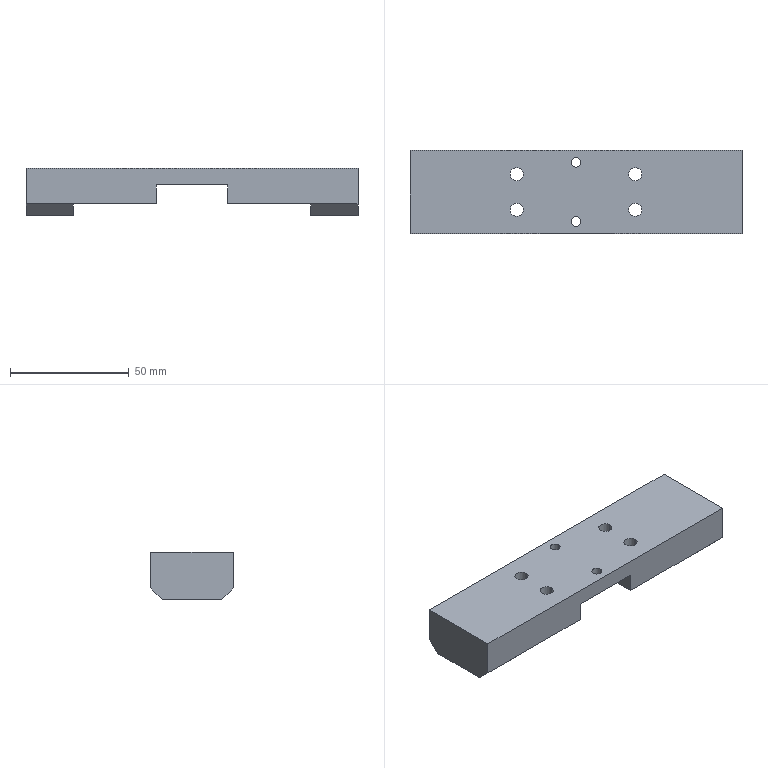Part | STEP file | PN_0024 Rodless cylinder connecting plate | 1 solid | 42 faces | box 140 x 35 x 20 mm | volume 68524 mm3 | plane 22 | cylinder 20 | commonest cylinder face diameters 5.5 x8 9 x8 4.2 x4